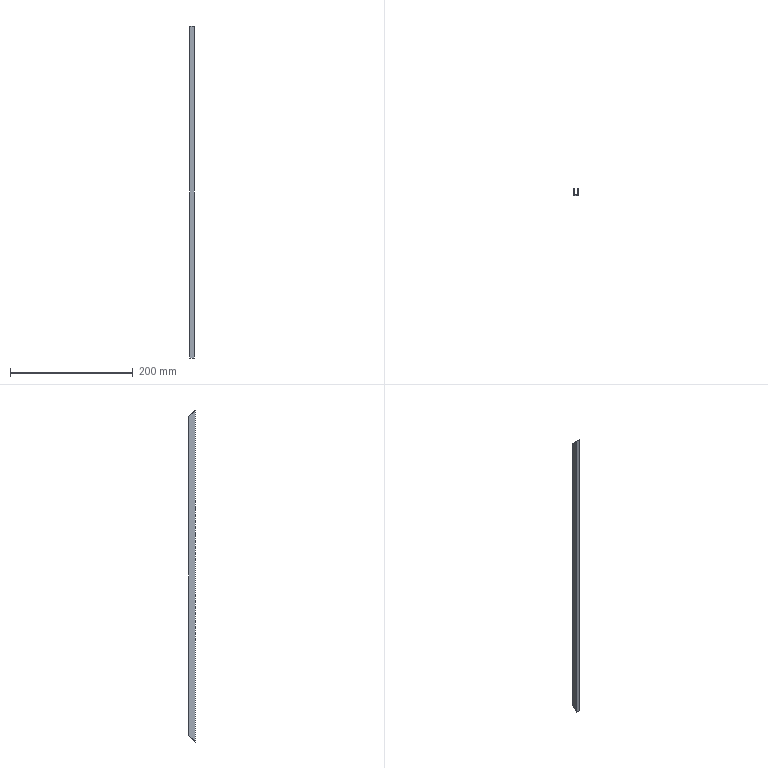Part | STEP file | Friction strip L542 | 1 solid | 10 faces | box 7 x 11 x 542 mm | volume 14387 mm3 | plane 10
STEP:
#1=CARTESIAN_POINT('',(0.,0.,0.));
#2=DIRECTION('',(0.,0.,1.));
#3=DIRECTION('',(1.,0.,0.));
#4=AXIS2_PLACEMENT_3D('',#1,#2,#3);
#5=CARTESIAN_POINT('',(3.5,0.,542.));
#6=VERTEX_POINT('',#5);
#7=CARTESIAN_POINT('',(3.5,0.,0.));
#8=VERTEX_POINT('',#7);
#9=CARTESIAN_POINT('',(3.5,0.,542.));
#10=DIRECTION('',(0.,0.,-1.));
#11=VECTOR('',#10,1.);
#12=LINE('',#9,#11);
#13=CARTESIAN_POINT('',(3.5,0.,542.));
#14=DIRECTION('',(-1.,0.,0.));
#15=DIRECTION('',(0.,-1.,0.));
#16=AXIS2_PLACEMENT_3D('',#13,#14,#15);
#17=PLANE('',#16);
#18=CARTESIAN_POINT('',(0.,0.));
#19=DIRECTION('',(0.,-1.));
#20=VECTOR('',#19,1.);
#21=LINE('',#18,#20);
#22=(GEOMETRIC_REPRESENTATION_CONTEXT(2)PARAMETRIC_REPRESENTATION_CONTEXT()REPRESENTATION_CONTEXT('',''));
#23=DEFINITIONAL_REPRESENTATION('',(#21),#22);
#24=PCURVE('',#17,#23);
#25=CARTESIAN_POINT('',(-3.5,0.,542.));
#26=DIRECTION('',(0.,1.,0.));
#27=DIRECTION('',(0.,0.,1.));
#28=AXIS2_PLACEMENT_3D('',#25,#26,#27);
#29=PLANE('',#28);
#30=CARTESIAN_POINT('',(0.,7.));
#31=DIRECTION('',(-1.,0.));
#32=VECTOR('',#31,1.);
#33=LINE('',#30,#32);
#34=(GEOMETRIC_REPRESENTATION_CONTEXT(2)PARAMETRIC_REPRESENTATION_CONTEXT()REPRESENTATION_CONTEXT('',''));
#35=DEFINITIONAL_REPRESENTATION('',(#33),#34);
#36=PCURVE('',#29,#35);
#37=SURFACE_CURVE('',#12,(#24,#36),.PCURVE_S1.);
#38=EDGE_CURVE('',#6,#8,#37,.T.);
#39=ORIENTED_EDGE('',*,*,#38,.T.);
#40=CARTESIAN_POINT('',(3.5,11.,11.));
#41=VERTEX_POINT('',#40);
#42=CARTESIAN_POINT('',(3.5,0.,0.));
#43=DIRECTION('',(0.,0.7071,0.7071));
#44=VECTOR('',#43,1.);
#45=LINE('',#42,#44);
#46=CARTESIAN_POINT('',(0.,-542.));
#47=DIRECTION('',(-0.7071,0.7071));
#48=VECTOR('',#47,1.);
#49=LINE('',#46,#48);
#50=(GEOMETRIC_REPRESENTATION_CONTEXT(2)PARAMETRIC_REPRESENTATION_CONTEXT()REPRESENTATION_CONTEXT('',''));
#51=DEFINITIONAL_REPRESENTATION('',(#49),#50);
#52=PCURVE('',#17,#51);
#53=CARTESIAN_POINT('',(3.5,0.,0.));
#54=DIRECTION('',(0.,-0.7071,0.7071));
#55=DIRECTION('',(0.,-0.7071,-0.7071));
#56=AXIS2_PLACEMENT_3D('',#53,#54,#55);
#57=PLANE('',#56);
#58=CARTESIAN_POINT('',(0.,0.));
#59=DIRECTION('',(-1.,0.));
#60=VECTOR('',#59,1.);
#61=LINE('',#58,#60);
#62=(GEOMETRIC_REPRESENTATION_CONTEXT(2)PARAMETRIC_REPRESENTATION_CONTEXT()REPRESENTATION_CONTEXT('',''));
#63=DEFINITIONAL_REPRESENTATION('',(#61),#62);
#64=PCURVE('',#57,#63);
#65=SURFACE_CURVE('',#45,(#52,#64),.PCURVE_S1.);
#66=EDGE_CURVE('',#8,#41,#65,.T.);
#67=ORIENTED_EDGE('',*,*,#66,.T.);
#68=CARTESIAN_POINT('',(3.5,11.,531.));
#69=VERTEX_POINT('',#68);
#70=CARTESIAN_POINT('',(3.5,11.,542.));
#71=DIRECTION('',(0.,0.,-1.));
#72=VECTOR('',#71,1.);
#73=LINE('',#70,#72);
#74=CARTESIAN_POINT('',(-11.,0.));
#75=DIRECTION('',(0.,-1.));
#76=VECTOR('',#75,1.);
#77=LINE('',#74,#76);
#78=(GEOMETRIC_REPRESENTATION_CONTEXT(2)PARAMETRIC_REPRESENTATION_CONTEXT()REPRESENTATION_CONTEXT('',''));
#79=DEFINITIONAL_REPRESENTATION('',(#77),#78);
#80=PCURVE('',#17,#79);
#81=CARTESIAN_POINT('',(2.5,11.,542.));
#82=DIRECTION('',(0.,1.,0.));
#83=DIRECTION('',(0.,0.,1.));
#84=AXIS2_PLACEMENT_3D('',#81,#82,#83);
#85=PLANE('',#84);
#86=CARTESIAN_POINT('',(0.,1.));
#87=DIRECTION('',(-1.,0.));
#88=VECTOR('',#87,1.);
#89=LINE('',#86,#88);
#90=(GEOMETRIC_REPRESENTATION_CONTEXT(2)PARAMETRIC_REPRESENTATION_CONTEXT()REPRESENTATION_CONTEXT('',''));
#91=DEFINITIONAL_REPRESENTATION('',(#89),#90);
#92=PCURVE('',#85,#91);
#93=SURFACE_CURVE('',#73,(#80,#92),.PCURVE_S1.);
#94=EDGE_CURVE('',#69,#41,#93,.T.);
#95=ORIENTED_EDGE('',*,*,#94,.F.);
#96=CARTESIAN_POINT('',(3.5,0.,542.));
#97=DIRECTION('',(0.,-0.7071,0.7071));
#98=VECTOR('',#97,1.);
#99=LINE('',#96,#98);
#100=CARTESIAN_POINT('',(0.,0.));
#101=DIRECTION('',(0.7071,0.7071));
#102=VECTOR('',#101,1.);
#103=LINE('',#100,#102);
#104=(GEOMETRIC_REPRESENTATION_CONTEXT(2)PARAMETRIC_REPRESENTATION_CONTEXT()REPRESENTATION_CONTEXT('',''));
#105=DEFINITIONAL_REPRESENTATION('',(#103),#104);
#106=PCURVE('',#17,#105);
#107=CARTESIAN_POINT('',(3.5,0.,542.));
#108=DIRECTION('',(0.,-0.7071,-0.7071));
#109=DIRECTION('',(0.,0.7071,-0.7071));
#110=AXIS2_PLACEMENT_3D('',#107,#108,#109);
#111=PLANE('',#110);
#112=CARTESIAN_POINT('',(0.,0.));
#113=DIRECTION('',(-1.,0.));
#114=VECTOR('',#113,1.);
#115=LINE('',#112,#114);
#116=(GEOMETRIC_REPRESENTATION_CONTEXT(2)PARAMETRIC_REPRESENTATION_CONTEXT()REPRESENTATION_CONTEXT('',''));
#117=DEFINITIONAL_REPRESENTATION('',(#115),#116);
#118=PCURVE('',#111,#117);
#119=SURFACE_CURVE('',#99,(#106,#118),.PCURVE_S1.);
#120=EDGE_CURVE('',#69,#6,#119,.T.);
#121=ORIENTED_EDGE('',*,*,#120,.T.);
#122=EDGE_LOOP('',(#39,#67,#95,#121));
#123=FACE_BOUND('',#122,.T.);
#124=ADVANCED_FACE('',(#123),#17,.F.);
#125=CARTESIAN_POINT('',(2.5,11.,11.));
#126=VERTEX_POINT('',#125);
#127=CARTESIAN_POINT('',(3.5,11.,11.));
#128=DIRECTION('',(-1.,0.,0.));
#129=VECTOR('',#128,1.);
#130=LINE('',#127,#129);
#131=CARTESIAN_POINT('',(-531.,1.));
#132=DIRECTION('',(0.,-1.));
#133=VECTOR('',#132,1.);
#134=LINE('',#131,#133);
#135=(GEOMETRIC_REPRESENTATION_CONTEXT(2)PARAMETRIC_REPRESENTATION_CONTEXT()REPRESENTATION_CONTEXT('',''));
#136=DEFINITIONAL_REPRESENTATION('',(#134),#135);
#137=PCURVE('',#85,#136);
#138=CARTESIAN_POINT('',(-15.556,0.));
#139=DIRECTION('',(0.,-1.));
#140=VECTOR('',#139,1.);
#141=LINE('',#138,#140);
#142=(GEOMETRIC_REPRESENTATION_CONTEXT(2)PARAMETRIC_REPRESENTATION_CONTEXT()REPRESENTATION_CONTEXT('',''));
#143=DEFINITIONAL_REPRESENTATION('',(#141),#142);
#144=PCURVE('',#57,#143);
#145=SURFACE_CURVE('',#130,(#137,#144),.PCURVE_S1.);
#146=EDGE_CURVE('',#41,#126,#145,.T.);
#147=ORIENTED_EDGE('',*,*,#146,.T.);
#148=CARTESIAN_POINT('',(2.5,11.,531.));
#149=VERTEX_POINT('',#148);
#150=CARTESIAN_POINT('',(2.5,11.,542.));
#151=DIRECTION('',(0.,0.,-1.));
#152=VECTOR('',#151,1.);
#153=LINE('',#150,#152);
#154=CARTESIAN_POINT('',(0.,0.));
#155=DIRECTION('',(-1.,0.));
#156=VECTOR('',#155,1.);
#157=LINE('',#154,#156);
#158=(GEOMETRIC_REPRESENTATION_CONTEXT(2)PARAMETRIC_REPRESENTATION_CONTEXT()REPRESENTATION_CONTEXT('',''));
#159=DEFINITIONAL_REPRESENTATION('',(#157),#158);
#160=PCURVE('',#85,#159);
#161=CARTESIAN_POINT('',(2.5,0.,542.));
#162=DIRECTION('',(-1.,0.,0.));
#163=DIRECTION('',(0.,-1.,0.));
#164=AXIS2_PLACEMENT_3D('',#161,#162,#163);
#165=PLANE('',#164);
#166=CARTESIAN_POINT('',(-11.,0.));
#167=DIRECTION('',(0.,-1.));
#168=VECTOR('',#167,1.);
#169=LINE('',#166,#168);
#170=(GEOMETRIC_REPRESENTATION_CONTEXT(2)PARAMETRIC_REPRESENTATION_CONTEXT()REPRESENTATION_CONTEXT('',''));
#171=DEFINITIONAL_REPRESENTATION('',(#169),#170);
#172=PCURVE('',#165,#171);
#173=SURFACE_CURVE('',#153,(#160,#172),.PCURVE_S1.);
#174=EDGE_CURVE('',#149,#126,#173,.T.);
#175=ORIENTED_EDGE('',*,*,#174,.F.);
#176=CARTESIAN_POINT('',(3.5,11.,531.));
#177=DIRECTION('',(-1.,0.,0.));
#178=VECTOR('',#177,1.);
#179=LINE('',#176,#178);
#180=CARTESIAN_POINT('',(-11.,1.));
#181=DIRECTION('',(0.,-1.));
#182=VECTOR('',#181,1.);
#183=LINE('',#180,#182);
#184=(GEOMETRIC_REPRESENTATION_CONTEXT(2)PARAMETRIC_REPRESENTATION_CONTEXT()REPRESENTATION_CONTEXT('',''));
#185=DEFINITIONAL_REPRESENTATION('',(#183),#184);
#186=PCURVE('',#85,#185);
#187=CARTESIAN_POINT('',(15.556,0.));
#188=DIRECTION('',(0.,-1.));
#189=VECTOR('',#188,1.);
#190=LINE('',#187,#189);
#191=(GEOMETRIC_REPRESENTATION_CONTEXT(2)PARAMETRIC_REPRESENTATION_CONTEXT()REPRESENTATION_CONTEXT('',''));
#192=DEFINITIONAL_REPRESENTATION('',(#190),#191);
#193=PCURVE('',#111,#192);
#194=SURFACE_CURVE('',#179,(#186,#193),.PCURVE_S1.);
#195=EDGE_CURVE('',#69,#149,#194,.T.);
#196=ORIENTED_EDGE('',*,*,#195,.F.);
#197=ORIENTED_EDGE('',*,*,#94,.T.);
#198=EDGE_LOOP('',(#147,#175,#196,#197));
#199=FACE_BOUND('',#198,.T.);
#200=ADVANCED_FACE('',(#199),#85,.T.);
#201=CARTESIAN_POINT('',(2.5,1.,1.));
#202=VERTEX_POINT('',#201);
#203=CARTESIAN_POINT('',(2.5,271.,271.));
#204=DIRECTION('',(0.,0.7071,0.7071));
#205=VECTOR('',#204,1.);
#206=LINE('',#203,#205);
#207=CARTESIAN_POINT('',(-271.,-271.));
#208=DIRECTION('',(-0.7071,0.7071));
#209=VECTOR('',#208,1.);
#210=LINE('',#207,#209);
#211=(GEOMETRIC_REPRESENTATION_CONTEXT(2)PARAMETRIC_REPRESENTATION_CONTEXT()REPRESENTATION_CONTEXT('',''));
#212=DEFINITIONAL_REPRESENTATION('',(#210),#211);
#213=PCURVE('',#165,#212);
#214=CARTESIAN_POINT('',(-383.252,-1.));
#215=DIRECTION('',(-1.,0.));
#216=VECTOR('',#215,1.);
#217=LINE('',#214,#216);
#218=(GEOMETRIC_REPRESENTATION_CONTEXT(2)PARAMETRIC_REPRESENTATION_CONTEXT()REPRESENTATION_CONTEXT('',''));
#219=DEFINITIONAL_REPRESENTATION('',(#217),#218);
#220=PCURVE('',#57,#219);
#221=SURFACE_CURVE('',#206,(#213,#220),.PCURVE_S1.);
#222=EDGE_CURVE('',#202,#126,#221,.T.);
#223=ORIENTED_EDGE('',*,*,#222,.F.);
#224=CARTESIAN_POINT('',(2.5,1.,541.));
#225=VERTEX_POINT('',#224);
#226=CARTESIAN_POINT('',(2.5,1.,542.));
#227=DIRECTION('',(0.,0.,-1.));
#228=VECTOR('',#227,1.);
#229=LINE('',#226,#228);
#230=CARTESIAN_POINT('',(-1.,0.));
#231=DIRECTION('',(0.,-1.));
#232=VECTOR('',#231,1.);
#233=LINE('',#230,#232);
#234=(GEOMETRIC_REPRESENTATION_CONTEXT(2)PARAMETRIC_REPRESENTATION_CONTEXT()REPRESENTATION_CONTEXT('',''));
#235=DEFINITIONAL_REPRESENTATION('',(#233),#234);
#236=PCURVE('',#165,#235);
#237=CARTESIAN_POINT('',(-3.5,1.,542.));
#238=DIRECTION('',(0.,1.,0.));
#239=DIRECTION('',(0.,0.,1.));
#240=AXIS2_PLACEMENT_3D('',#237,#238,#239);
#241=PLANE('',#240);
#242=CARTESIAN_POINT('',(0.,6.));
#243=DIRECTION('',(-1.,0.));
#244=VECTOR('',#243,1.);
#245=LINE('',#242,#244);
#246=(GEOMETRIC_REPRESENTATION_CONTEXT(2)PARAMETRIC_REPRESENTATION_CONTEXT()REPRESENTATION_CONTEXT('',''));
#247=DEFINITIONAL_REPRESENTATION('',(#245),#246);
#248=PCURVE('',#241,#247);
#249=SURFACE_CURVE('',#229,(#236,#248),.PCURVE_S1.);
#250=EDGE_CURVE('',#225,#202,#249,.T.);
#251=ORIENTED_EDGE('',*,*,#250,.F.);
#252=CARTESIAN_POINT('',(2.5,0.,542.));
#253=DIRECTION('',(0.,-0.7071,0.7071));
#254=VECTOR('',#253,1.);
#255=LINE('',#252,#254);
#256=CARTESIAN_POINT('',(0.,0.));
#257=DIRECTION('',(0.7071,0.7071));
#258=VECTOR('',#257,1.);
#259=LINE('',#256,#258);
#260=(GEOMETRIC_REPRESENTATION_CONTEXT(2)PARAMETRIC_REPRESENTATION_CONTEXT()REPRESENTATION_CONTEXT('',''));
#261=DEFINITIONAL_REPRESENTATION('',(#259),#260);
#262=PCURVE('',#165,#261);
#263=CARTESIAN_POINT('',(0.,-1.));
#264=DIRECTION('',(-1.,0.));
#265=VECTOR('',#264,1.);
#266=LINE('',#263,#265);
#267=(GEOMETRIC_REPRESENTATION_CONTEXT(2)PARAMETRIC_REPRESENTATION_CONTEXT()REPRESENTATION_CONTEXT('',''));
#268=DEFINITIONAL_REPRESENTATION('',(#266),#267);
#269=PCURVE('',#111,#268);
#270=SURFACE_CURVE('',#255,(#262,#269),.PCURVE_S1.);
#271=EDGE_CURVE('',#149,#225,#270,.T.);
#272=ORIENTED_EDGE('',*,*,#271,.F.);
#273=ORIENTED_EDGE('',*,*,#174,.T.);
#274=EDGE_LOOP('',(#223,#251,#272,#273));
#275=FACE_BOUND('',#274,.T.);
#276=ADVANCED_FACE('',(#275),#165,.T.);
#277=CARTESIAN_POINT('',(-2.5,1.,1.));
#278=VERTEX_POINT('',#277);
#279=CARTESIAN_POINT('',(-3.5,1.,1.));
#280=DIRECTION('',(1.,0.,0.));
#281=VECTOR('',#280,1.);
#282=LINE('',#279,#281);
#283=CARTESIAN_POINT('',(-541.,0.));
#284=DIRECTION('',(0.,1.));
#285=VECTOR('',#284,1.);
#286=LINE('',#283,#285);
#287=(GEOMETRIC_REPRESENTATION_CONTEXT(2)PARAMETRIC_REPRESENTATION_CONTEXT()REPRESENTATION_CONTEXT('',''));
#288=DEFINITIONAL_REPRESENTATION('',(#286),#287);
#289=PCURVE('',#241,#288);
#290=CARTESIAN_POINT('',(-1.414,-7.));
#291=DIRECTION('',(0.,1.));
#292=VECTOR('',#291,1.);
#293=LINE('',#290,#292);
#294=(GEOMETRIC_REPRESENTATION_CONTEXT(2)PARAMETRIC_REPRESENTATION_CONTEXT()REPRESENTATION_CONTEXT('',''));
#295=DEFINITIONAL_REPRESENTATION('',(#293),#294);
#296=PCURVE('',#57,#295);
#297=SURFACE_CURVE('',#282,(#289,#296),.PCURVE_S1.);
#298=EDGE_CURVE('',#278,#202,#297,.T.);
#299=ORIENTED_EDGE('',*,*,#298,.F.);
#300=CARTESIAN_POINT('',(-2.5,1.,541.));
#301=VERTEX_POINT('',#300);
#302=CARTESIAN_POINT('',(-2.5,1.,542.));
#303=DIRECTION('',(0.,0.,-1.));
#304=VECTOR('',#303,1.);
#305=LINE('',#302,#304);
#306=CARTESIAN_POINT('',(0.,1.));
#307=DIRECTION('',(-1.,0.));
#308=VECTOR('',#307,1.);
#309=LINE('',#306,#308);
#310=(GEOMETRIC_REPRESENTATION_CONTEXT(2)PARAMETRIC_REPRESENTATION_CONTEXT()REPRESENTATION_CONTEXT('',''));
#311=DEFINITIONAL_REPRESENTATION('',(#309),#310);
#312=PCURVE('',#241,#311);
#313=CARTESIAN_POINT('',(-2.5,11.,542.));
#314=DIRECTION('',(1.,0.,0.));
#315=DIRECTION('',(0.,1.,0.));
#316=AXIS2_PLACEMENT_3D('',#313,#314,#315);
#317=PLANE('',#316);
#318=CARTESIAN_POINT('',(-10.,0.));
#319=DIRECTION('',(0.,-1.));
#320=VECTOR('',#319,1.);
#321=LINE('',#318,#320);
#322=(GEOMETRIC_REPRESENTATION_CONTEXT(2)PARAMETRIC_REPRESENTATION_CONTEXT()REPRESENTATION_CONTEXT('',''));
#323=DEFINITIONAL_REPRESENTATION('',(#321),#322);
#324=PCURVE('',#317,#323);
#325=SURFACE_CURVE('',#305,(#312,#324),.PCURVE_S1.);
#326=EDGE_CURVE('',#301,#278,#325,.T.);
#327=ORIENTED_EDGE('',*,*,#326,.F.);
#328=CARTESIAN_POINT('',(-3.5,1.,541.));
#329=DIRECTION('',(-1.,0.,0.));
#330=VECTOR('',#329,1.);
#331=LINE('',#328,#330);
#332=CARTESIAN_POINT('',(-1.,0.));
#333=DIRECTION('',(0.,-1.));
#334=VECTOR('',#333,1.);
#335=LINE('',#332,#334);
#336=(GEOMETRIC_REPRESENTATION_CONTEXT(2)PARAMETRIC_REPRESENTATION_CONTEXT()REPRESENTATION_CONTEXT('',''));
#337=DEFINITIONAL_REPRESENTATION('',(#335),#336);
#338=PCURVE('',#241,#337);
#339=CARTESIAN_POINT('',(1.414,-7.));
#340=DIRECTION('',(0.,-1.));
#341=VECTOR('',#340,1.);
#342=LINE('',#339,#341);
#343=(GEOMETRIC_REPRESENTATION_CONTEXT(2)PARAMETRIC_REPRESENTATION_CONTEXT()REPRESENTATION_CONTEXT('',''));
#344=DEFINITIONAL_REPRESENTATION('',(#342),#343);
#345=PCURVE('',#111,#344);
#346=SURFACE_CURVE('',#331,(#338,#345),.PCURVE_S1.);
#347=EDGE_CURVE('',#225,#301,#346,.T.);
#348=ORIENTED_EDGE('',*,*,#347,.F.);
#349=ORIENTED_EDGE('',*,*,#250,.T.);
#350=EDGE_LOOP('',(#299,#327,#348,#349));
#351=FACE_BOUND('',#350,.T.);
#352=ADVANCED_FACE('',(#351),#241,.T.);
#353=CARTESIAN_POINT('',(-2.5,11.,11.));
#354=VERTEX_POINT('',#353);
#355=CARTESIAN_POINT('',(-2.5,276.5,276.5));
#356=DIRECTION('',(0.,-0.7071,-0.7071));
#357=VECTOR('',#356,1.);
#358=LINE('',#355,#357);
#359=CARTESIAN_POINT('',(265.5,-265.5));
#360=DIRECTION('',(-0.7071,-0.7071));
#361=VECTOR('',#360,1.);
#362=LINE('',#359,#361);
#363=(GEOMETRIC_REPRESENTATION_CONTEXT(2)PARAMETRIC_REPRESENTATION_CONTEXT()REPRESENTATION_CONTEXT('',''));
#364=DEFINITIONAL_REPRESENTATION('',(#362),#363);
#365=PCURVE('',#317,#364);
#366=CARTESIAN_POINT('',(-391.03,-6.));
#367=DIRECTION('',(1.,0.));
#368=VECTOR('',#367,1.);
#369=LINE('',#366,#368);
#370=(GEOMETRIC_REPRESENTATION_CONTEXT(2)PARAMETRIC_REPRESENTATION_CONTEXT()REPRESENTATION_CONTEXT('',''));
#371=DEFINITIONAL_REPRESENTATION('',(#369),#370);
#372=PCURVE('',#57,#371);
#373=SURFACE_CURVE('',#358,(#365,#372),.PCURVE_S1.);
#374=EDGE_CURVE('',#354,#278,#373,.T.);
#375=ORIENTED_EDGE('',*,*,#374,.F.);
#376=CARTESIAN_POINT('',(-2.5,11.,531.));
#377=VERTEX_POINT('',#376);
#378=CARTESIAN_POINT('',(-2.5,11.,542.));
#379=DIRECTION('',(0.,0.,-1.));
#380=VECTOR('',#379,1.);
#381=LINE('',#378,#380);
#382=CARTESIAN_POINT('',(0.,0.));
#383=DIRECTION('',(0.,-1.));
#384=VECTOR('',#383,1.);
#385=LINE('',#382,#384);
#386=(GEOMETRIC_REPRESENTATION_CONTEXT(2)PARAMETRIC_REPRESENTATION_CONTEXT()REPRESENTATION_CONTEXT('',''));
#387=DEFINITIONAL_REPRESENTATION('',(#385),#386);
#388=PCURVE('',#317,#387);
#389=CARTESIAN_POINT('',(-3.5,11.,542.));
#390=DIRECTION('',(0.,1.,0.));
#391=DIRECTION('',(0.,0.,1.));
#392=AXIS2_PLACEMENT_3D('',#389,#390,#391);
#393=PLANE('',#392);
#394=CARTESIAN_POINT('',(0.,1.));
#395=DIRECTION('',(-1.,0.));
#396=VECTOR('',#395,1.);
#397=LINE('',#394,#396);
#398=(GEOMETRIC_REPRESENTATION_CONTEXT(2)PARAMETRIC_REPRESENTATION_CONTEXT()REPRESENTATION_CONTEXT('',''));
#399=DEFINITIONAL_REPRESENTATION('',(#397),#398);
#400=PCURVE('',#393,#399);
#401=SURFACE_CURVE('',#381,(#388,#400),.PCURVE_S1.);
#402=EDGE_CURVE('',#377,#354,#401,.T.);
#403=ORIENTED_EDGE('',*,*,#402,.F.);
#404=CARTESIAN_POINT('',(-2.5,5.5,536.5));
#405=DIRECTION('',(0.,0.7071,-0.7071));
#406=VECTOR('',#405,1.);
#407=LINE('',#404,#406);
#408=CARTESIAN_POINT('',(-5.5,-5.5));
#409=DIRECTION('',(0.7071,-0.7071));
#410=VECTOR('',#409,1.);
#411=LINE('',#408,#410);
#412=(GEOMETRIC_REPRESENTATION_CONTEXT(2)PARAMETRIC_REPRESENTATION_CONTEXT()REPRESENTATION_CONTEXT('',''));
#413=DEFINITIONAL_REPRESENTATION('',(#411),#412);
#414=PCURVE('',#317,#413);
#415=CARTESIAN_POINT('',(7.778,-6.));
#416=DIRECTION('',(1.,0.));
#417=VECTOR('',#416,1.);
#418=LINE('',#415,#417);
#419=(GEOMETRIC_REPRESENTATION_CONTEXT(2)PARAMETRIC_REPRESENTATION_CONTEXT()REPRESENTATION_CONTEXT('',''));
#420=DEFINITIONAL_REPRESENTATION('',(#418),#419);
#421=PCURVE('',#111,#420);
#422=SURFACE_CURVE('',#407,(#414,#421),.PCURVE_S1.);
#423=EDGE_CURVE('',#301,#377,#422,.T.);
#424=ORIENTED_EDGE('',*,*,#423,.F.);
#425=ORIENTED_EDGE('',*,*,#326,.T.);
#426=EDGE_LOOP('',(#375,#403,#424,#425));
#427=FACE_BOUND('',#426,.T.);
#428=ADVANCED_FACE('',(#427),#317,.T.);
#429=CARTESIAN_POINT('',(-3.5,11.,11.));
#430=VERTEX_POINT('',#429);
#431=CARTESIAN_POINT('',(3.5,11.,11.));
#432=DIRECTION('',(-1.,0.,0.));
#433=VECTOR('',#432,1.);
#434=LINE('',#431,#433);
#435=CARTESIAN_POINT('',(-531.,7.));
#436=DIRECTION('',(0.,-1.));
#437=VECTOR('',#436,1.);
#438=LINE('',#435,#437);
#439=(GEOMETRIC_REPRESENTATION_CONTEXT(2)PARAMETRIC_REPRESENTATION_CONTEXT()REPRESENTATION_CONTEXT('',''));
#440=DEFINITIONAL_REPRESENTATION('',(#438),#439);
#441=PCURVE('',#393,#440);
#442=CARTESIAN_POINT('',(-15.556,0.));
#443=DIRECTION('',(0.,-1.));
#444=VECTOR('',#443,1.);
#445=LINE('',#442,#444);
#446=(GEOMETRIC_REPRESENTATION_CONTEXT(2)PARAMETRIC_REPRESENTATION_CONTEXT()REPRESENTATION_CONTEXT('',''));
#447=DEFINITIONAL_REPRESENTATION('',(#445),#446);
#448=PCURVE('',#57,#447);
#449=SURFACE_CURVE('',#434,(#441,#448),.PCURVE_S1.);
#450=EDGE_CURVE('',#354,#430,#449,.T.);
#451=ORIENTED_EDGE('',*,*,#450,.T.);
#452=CARTESIAN_POINT('',(-3.5,11.,531.));
#453=VERTEX_POINT('',#452);
#454=CARTESIAN_POINT('',(-3.5,11.,542.));
#455=DIRECTION('',(0.,0.,-1.));
#456=VECTOR('',#455,1.);
#457=LINE('',#454,#456);
#458=CARTESIAN_POINT('',(0.,0.));
#459=DIRECTION('',(-1.,0.));
#460=VECTOR('',#459,1.);
#461=LINE('',#458,#460);
#462=(GEOMETRIC_REPRESENTATION_CONTEXT(2)PARAMETRIC_REPRESENTATION_CONTEXT()REPRESENTATION_CONTEXT('',''));
#463=DEFINITIONAL_REPRESENTATION('',(#461),#462);
#464=PCURVE('',#393,#463);
#465=CARTESIAN_POINT('',(-3.5,11.,542.));
#466=DIRECTION('',(1.,0.,0.));
#467=DIRECTION('',(0.,1.,0.));
#468=AXIS2_PLACEMENT_3D('',#465,#466,#467);
#469=PLANE('',#468);
#470=CARTESIAN_POINT('',(0.,0.));
#471=DIRECTION('',(0.,-1.));
#472=VECTOR('',#471,1.);
#473=LINE('',#470,#472);
#474=(GEOMETRIC_REPRESENTATION_CONTEXT(2)PARAMETRIC_REPRESENTATION_CONTEXT()REPRESENTATION_CONTEXT('',''));
#475=DEFINITIONAL_REPRESENTATION('',(#473),#474);
#476=PCURVE('',#469,#475);
#477=SURFACE_CURVE('',#457,(#464,#476),.PCURVE_S1.);
#478=EDGE_CURVE('',#453,#430,#477,.T.);
#479=ORIENTED_EDGE('',*,*,#478,.F.);
#480=CARTESIAN_POINT('',(3.5,11.,531.));
#481=DIRECTION('',(-1.,0.,0.));
#482=VECTOR('',#481,1.);
#483=LINE('',#480,#482);
#484=CARTESIAN_POINT('',(-11.,7.));
#485=DIRECTION('',(0.,-1.));
#486=VECTOR('',#485,1.);
#487=LINE('',#484,#486);
#488=(GEOMETRIC_REPRESENTATION_CONTEXT(2)PARAMETRIC_REPRESENTATION_CONTEXT()REPRESENTATION_CONTEXT('',''));
#489=DEFINITIONAL_REPRESENTATION('',(#487),#488);
#490=PCURVE('',#393,#489);
#491=CARTESIAN_POINT('',(15.556,0.));
#492=DIRECTION('',(0.,-1.));
#493=VECTOR('',#492,1.);
#494=LINE('',#491,#493);
#495=(GEOMETRIC_REPRESENTATION_CONTEXT(2)PARAMETRIC_REPRESENTATION_CONTEXT()REPRESENTATION_CONTEXT('',''));
#496=DEFINITIONAL_REPRESENTATION('',(#494),#495);
#497=PCURVE('',#111,#496);
#498=SURFACE_CURVE('',#483,(#490,#497),.PCURVE_S1.);
#499=EDGE_CURVE('',#377,#453,#498,.T.);
#500=ORIENTED_EDGE('',*,*,#499,.F.);
#501=ORIENTED_EDGE('',*,*,#402,.T.);
#502=EDGE_LOOP('',(#451,#479,#500,#501));
#503=FACE_BOUND('',#502,.T.);
#504=ADVANCED_FACE('',(#503),#393,.T.);
#505=ORIENTED_EDGE('',*,*,#478,.T.);
#506=CARTESIAN_POINT('',(-3.5,0.,0.));
#507=VERTEX_POINT('',#506);
#508=CARTESIAN_POINT('',(-3.5,0.,0.));
#509=DIRECTION('',(0.,0.7071,0.7071));
#510=VECTOR('',#509,1.);
#511=LINE('',#508,#510);
#512=CARTESIAN_POINT('',(-11.,-542.));
#513=DIRECTION('',(0.7071,0.7071));
#514=VECTOR('',#513,1.);
#515=LINE('',#512,#514);
#516=(GEOMETRIC_REPRESENTATION_CONTEXT(2)PARAMETRIC_REPRESENTATION_CONTEXT()REPRESENTATION_CONTEXT('',''));
#517=DEFINITIONAL_REPRESENTATION('',(#515),#516);
#518=PCURVE('',#469,#517);
#519=CARTESIAN_POINT('',(0.,-7.));
#520=DIRECTION('',(-1.,0.));
#521=VECTOR('',#520,1.);
#522=LINE('',#519,#521);
#523=(GEOMETRIC_REPRESENTATION_CONTEXT(2)PARAMETRIC_REPRESENTATION_CONTEXT()REPRESENTATION_CONTEXT('',''));
#524=DEFINITIONAL_REPRESENTATION('',(#522),#523);
#525=PCURVE('',#57,#524);
#526=SURFACE_CURVE('',#511,(#518,#525),.PCURVE_S1.);
#527=EDGE_CURVE('',#507,#430,#526,.T.);
#528=ORIENTED_EDGE('',*,*,#527,.F.);
#529=CARTESIAN_POINT('',(-3.5,0.,542.));
#530=VERTEX_POINT('',#529);
#531=CARTESIAN_POINT('',(-3.5,0.,542.));
#532=DIRECTION('',(0.,0.,-1.));
#533=VECTOR('',#532,1.);
#534=LINE('',#531,#533);
#535=CARTESIAN_POINT('',(-11.,0.));
#536=DIRECTION('',(0.,-1.));
#537=VECTOR('',#536,1.);
#538=LINE('',#535,#537);
#539=(GEOMETRIC_REPRESENTATION_CONTEXT(2)PARAMETRIC_REPRESENTATION_CONTEXT()REPRESENTATION_CONTEXT('',''));
#540=DEFINITIONAL_REPRESENTATION('',(#538),#539);
#541=PCURVE('',#469,#540);
#542=CARTESIAN_POINT('',(0.,0.));
#543=DIRECTION('',(-1.,0.));
#544=VECTOR('',#543,1.);
#545=LINE('',#542,#544);
#546=(GEOMETRIC_REPRESENTATION_CONTEXT(2)PARAMETRIC_REPRESENTATION_CONTEXT()REPRESENTATION_CONTEXT('',''));
#547=DEFINITIONAL_REPRESENTATION('',(#545),#546);
#548=PCURVE('',#29,#547);
#549=SURFACE_CURVE('',#534,(#541,#548),.PCURVE_S1.);
#550=EDGE_CURVE('',#530,#507,#549,.T.);
#551=ORIENTED_EDGE('',*,*,#550,.F.);
#552=CARTESIAN_POINT('',(-3.5,0.,542.));
#553=DIRECTION('',(0.,-0.7071,0.7071));
#554=VECTOR('',#553,1.);
#555=LINE('',#552,#554);
#556=CARTESIAN_POINT('',(-11.,0.));
#557=DIRECTION('',(-0.7071,0.7071));
#558=VECTOR('',#557,1.);
#559=LINE('',#556,#558);
#560=(GEOMETRIC_REPRESENTATION_CONTEXT(2)PARAMETRIC_REPRESENTATION_CONTEXT()REPRESENTATION_CONTEXT('',''));
#561=DEFINITIONAL_REPRESENTATION('',(#559),#560);
#562=PCURVE('',#469,#561);
#563=CARTESIAN_POINT('',(0.,-7.));
#564=DIRECTION('',(-1.,0.));
#565=VECTOR('',#564,1.);
#566=LINE('',#563,#565);
#567=(GEOMETRIC_REPRESENTATION_CONTEXT(2)PARAMETRIC_REPRESENTATION_CONTEXT()REPRESENTATION_CONTEXT('',''));
#568=DEFINITIONAL_REPRESENTATION('',(#566),#567);
#569=PCURVE('',#111,#568);
#570=SURFACE_CURVE('',#555,(#562,#569),.PCURVE_S1.);
#571=EDGE_CURVE('',#453,#530,#570,.T.);
#572=ORIENTED_EDGE('',*,*,#571,.F.);
#573=EDGE_LOOP('',(#505,#528,#551,#572));
#574=FACE_BOUND('',#573,.T.);
#575=ADVANCED_FACE('',(#574),#469,.F.);
#576=CARTESIAN_POINT('',(-3.5,0.,0.));
#577=DIRECTION('',(1.,0.,0.));
#578=VECTOR('',#577,1.);
#579=LINE('',#576,#578);
#580=CARTESIAN_POINT('',(-542.,0.));
#581=DIRECTION('',(0.,1.));
#582=VECTOR('',#581,1.);
#583=LINE('',#580,#582);
#584=(GEOMETRIC_REPRESENTATION_CONTEXT(2)PARAMETRIC_REPRESENTATION_CONTEXT()REPRESENTATION_CONTEXT('',''));
#585=DEFINITIONAL_REPRESENTATION('',(#583),#584);
#586=PCURVE('',#29,#585);
#587=CARTESIAN_POINT('',(0.,-7.));
#588=DIRECTION('',(0.,1.));
#589=VECTOR('',#588,1.);
#590=LINE('',#587,#589);
#591=(GEOMETRIC_REPRESENTATION_CONTEXT(2)PARAMETRIC_REPRESENTATION_CONTEXT()REPRESENTATION_CONTEXT('',''));
#592=DEFINITIONAL_REPRESENTATION('',(#590),#591);
#593=PCURVE('',#57,#592);
#594=SURFACE_CURVE('',#579,(#586,#593),.PCURVE_S1.);
#595=EDGE_CURVE('',#507,#8,#594,.T.);
#596=ORIENTED_EDGE('',*,*,#595,.T.);
#597=ORIENTED_EDGE('',*,*,#38,.F.);
#598=CARTESIAN_POINT('',(-3.5,0.,542.));
#599=DIRECTION('',(1.,0.,0.));
#600=VECTOR('',#599,1.);
#601=LINE('',#598,#600);
#602=CARTESIAN_POINT('',(0.,0.));
#603=DIRECTION('',(0.,1.));
#604=VECTOR('',#603,1.);
#605=LINE('',#602,#604);
#606=(GEOMETRIC_REPRESENTATION_CONTEXT(2)PARAMETRIC_REPRESENTATION_CONTEXT()REPRESENTATION_CONTEXT('',''));
#607=DEFINITIONAL_REPRESENTATION('',(#605),#606);
#608=PCURVE('',#29,#607);
#609=CARTESIAN_POINT('',(0.,-7.));
#610=DIRECTION('',(0.,1.));
#611=VECTOR('',#610,1.);
#612=LINE('',#609,#611);
#613=(GEOMETRIC_REPRESENTATION_CONTEXT(2)PARAMETRIC_REPRESENTATION_CONTEXT()REPRESENTATION_CONTEXT('',''));
#614=DEFINITIONAL_REPRESENTATION('',(#612),#613);
#615=PCURVE('',#111,#614);
#616=SURFACE_CURVE('',#601,(#608,#615),.PCURVE_S1.);
#617=EDGE_CURVE('',#530,#6,#616,.T.);
#618=ORIENTED_EDGE('',*,*,#617,.F.);
#619=ORIENTED_EDGE('',*,*,#550,.T.);
#620=EDGE_LOOP('',(#596,#597,#618,#619));
#621=FACE_BOUND('',#620,.T.);
#622=ADVANCED_FACE('',(#621),#29,.F.);
#623=ORIENTED_EDGE('',*,*,#271,.T.);
#624=ORIENTED_EDGE('',*,*,#347,.T.);
#625=ORIENTED_EDGE('',*,*,#423,.T.);
#626=ORIENTED_EDGE('',*,*,#499,.T.);
#627=ORIENTED_EDGE('',*,*,#571,.T.);
#628=ORIENTED_EDGE('',*,*,#617,.T.);
#629=ORIENTED_EDGE('',*,*,#120,.F.);
#630=ORIENTED_EDGE('',*,*,#195,.T.);
#631=EDGE_LOOP('',(#623,#624,#625,#626,#627,#628,#629,#630));
#632=FACE_BOUND('',#631,.T.);
#633=ADVANCED_FACE('',(#632),#111,.F.);
#634=ORIENTED_EDGE('',*,*,#222,.T.);
#635=ORIENTED_EDGE('',*,*,#146,.F.);
#636=ORIENTED_EDGE('',*,*,#66,.F.);
#637=ORIENTED_EDGE('',*,*,#595,.F.);
#638=ORIENTED_EDGE('',*,*,#527,.T.);
#639=ORIENTED_EDGE('',*,*,#450,.F.);
#640=ORIENTED_EDGE('',*,*,#374,.T.);
#641=ORIENTED_EDGE('',*,*,#298,.T.);
#642=EDGE_LOOP('',(#634,#635,#636,#637,#638,#639,#640,#641));
#643=FACE_BOUND('',#642,.T.);
#644=ADVANCED_FACE('',(#643),#57,.F.);
#645=CLOSED_SHELL('',(#124,#200,#276,#352,#428,#504,#575,#622,#633,#644));
#646=MANIFOLD_SOLID_BREP('',#645);
#647=(LENGTH_UNIT()NAMED_UNIT(*)SI_UNIT(.MILLI.,.METRE.));
#648=UNCERTAINTY_MEASURE_WITH_UNIT(LENGTH_MEASURE(0.0000001),#647,'','');
#649=(NAMED_UNIT(*)PLANE_ANGLE_UNIT()SI_UNIT($,.RADIAN.));
#650=(NAMED_UNIT(*)SI_UNIT($,.STERADIAN.)SOLID_ANGLE_UNIT());
#651=(GEOMETRIC_REPRESENTATION_CONTEXT(3)GLOBAL_UNCERTAINTY_ASSIGNED_CONTEXT((#648))GLOBAL_UNIT_ASSIGNED_CONTEXT((#647,#649,#650))REPRESENTATION_CONTEXT('',''));
#652=ADVANCED_BREP_SHAPE_REPRESENTATION('',(#4,#646),#651);